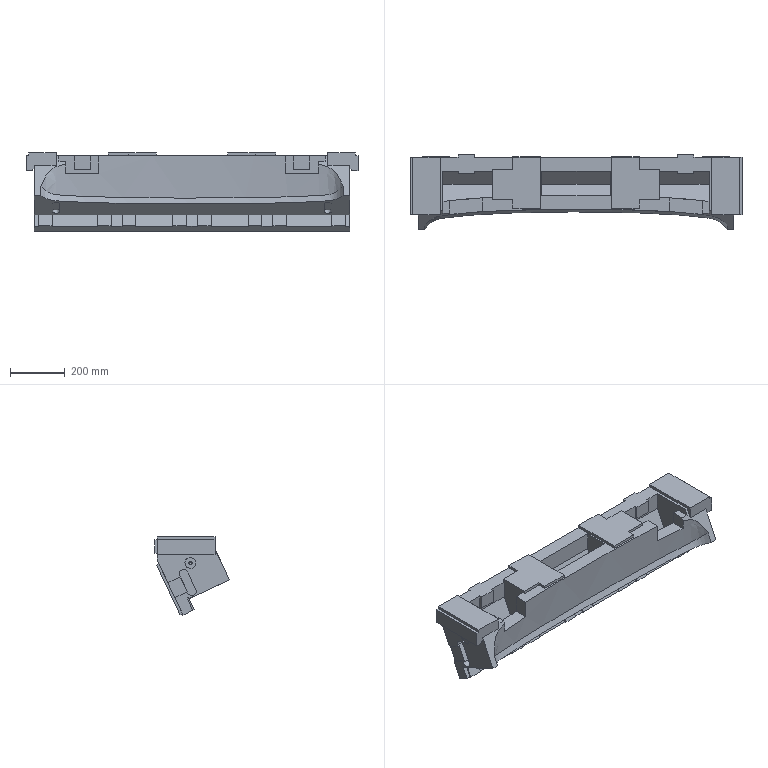Part | NX | features solid 2 | 1 solid | 197 faces | box 1210 x 272.322 x 284.802 mm | volume 38318164 mm3 | plane 173 | cylinder 12 | spline 10 | cone 2 | commonest cylinder face diameters 25 x4 32 x4 12 x2 40 x2